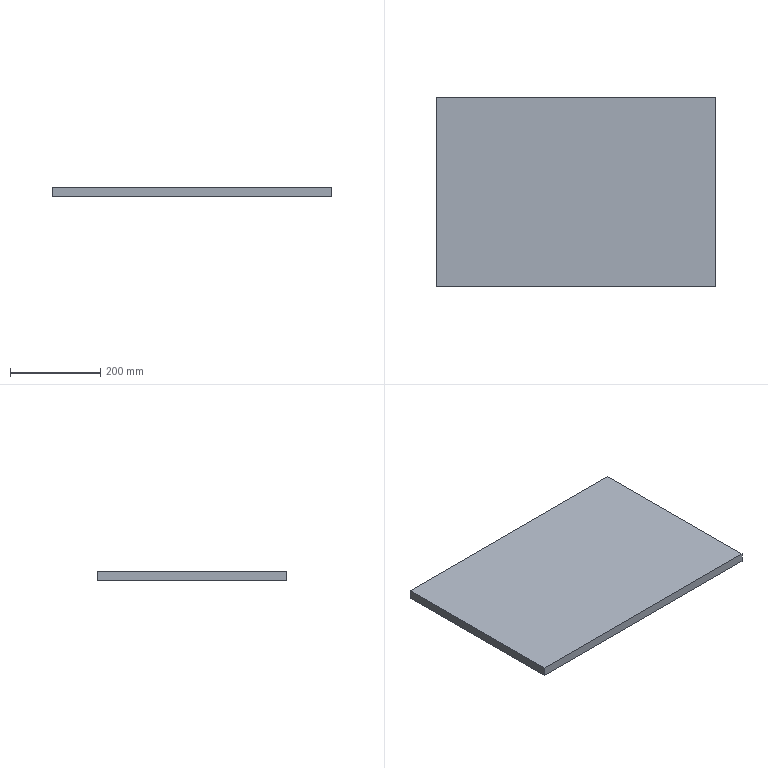Part | STEP file | Pad plate 2 | 1 solid | 6 faces | box 620 x 420 x 20 mm | volume 5208000 mm3 | plane 6
STEP:
#1=CARTESIAN_POINT('',(0.,0.,0.));
#2=DIRECTION('',(0.,0.,1.));
#3=DIRECTION('',(1.,0.,0.));
#4=AXIS2_PLACEMENT_3D('',#1,#2,#3);
#5=CARTESIAN_POINT('',(-310.,210.,20.));
#6=VERTEX_POINT('',#5);
#7=CARTESIAN_POINT('',(-310.,-210.,20.));
#8=VERTEX_POINT('',#7);
#9=CARTESIAN_POINT('',(-310.,0.,20.));
#10=DIRECTION('',(0.,-1.,0.));
#11=VECTOR('',#10,1.);
#12=LINE('',#9,#11);
#13=CARTESIAN_POINT('',(0.,0.,20.));
#14=DIRECTION('',(0.,0.,1.));
#15=DIRECTION('',(1.,0.,0.));
#16=AXIS2_PLACEMENT_3D('',#13,#14,#15);
#17=PLANE('',#16);
#18=CARTESIAN_POINT('',(-310.,0.));
#19=DIRECTION('',(0.,-1.));
#20=VECTOR('',#19,1.);
#21=LINE('',#18,#20);
#22=(GEOMETRIC_REPRESENTATION_CONTEXT(2)PARAMETRIC_REPRESENTATION_CONTEXT()REPRESENTATION_CONTEXT('',''));
#23=DEFINITIONAL_REPRESENTATION('',(#21),#22);
#24=PCURVE('',#17,#23);
#25=CARTESIAN_POINT('',(-310.,210.,20.));
#26=DIRECTION('',(1.,0.,0.));
#27=DIRECTION('',(0.,1.,0.));
#28=AXIS2_PLACEMENT_3D('',#25,#26,#27);
#29=PLANE('',#28);
#30=CARTESIAN_POINT('',(-210.,0.));
#31=DIRECTION('',(-1.,0.));
#32=VECTOR('',#31,1.);
#33=LINE('',#30,#32);
#34=(GEOMETRIC_REPRESENTATION_CONTEXT(2)PARAMETRIC_REPRESENTATION_CONTEXT()REPRESENTATION_CONTEXT('',''));
#35=DEFINITIONAL_REPRESENTATION('',(#33),#34);
#36=PCURVE('',#29,#35);
#37=SURFACE_CURVE('',#12,(#24,#36),.PCURVE_S1.);
#38=EDGE_CURVE('',#6,#8,#37,.T.);
#39=ORIENTED_EDGE('',*,*,#38,.T.);
#40=CARTESIAN_POINT('',(310.,-210.,20.));
#41=VERTEX_POINT('',#40);
#42=CARTESIAN_POINT('',(0.,-210.,20.));
#43=DIRECTION('',(1.,0.,0.));
#44=VECTOR('',#43,1.);
#45=LINE('',#42,#44);
#46=CARTESIAN_POINT('',(0.,-210.));
#47=DIRECTION('',(1.,0.));
#48=VECTOR('',#47,1.);
#49=LINE('',#46,#48);
#50=(GEOMETRIC_REPRESENTATION_CONTEXT(2)PARAMETRIC_REPRESENTATION_CONTEXT()REPRESENTATION_CONTEXT('',''));
#51=DEFINITIONAL_REPRESENTATION('',(#49),#50);
#52=PCURVE('',#17,#51);
#53=CARTESIAN_POINT('',(-310.,-210.,20.));
#54=DIRECTION('',(0.,1.,0.));
#55=DIRECTION('',(0.,0.,1.));
#56=AXIS2_PLACEMENT_3D('',#53,#54,#55);
#57=PLANE('',#56);
#58=CARTESIAN_POINT('',(0.,310.));
#59=DIRECTION('',(0.,1.));
#60=VECTOR('',#59,1.);
#61=LINE('',#58,#60);
#62=(GEOMETRIC_REPRESENTATION_CONTEXT(2)PARAMETRIC_REPRESENTATION_CONTEXT()REPRESENTATION_CONTEXT('',''));
#63=DEFINITIONAL_REPRESENTATION('',(#61),#62);
#64=PCURVE('',#57,#63);
#65=SURFACE_CURVE('',#45,(#52,#64),.PCURVE_S1.);
#66=EDGE_CURVE('',#8,#41,#65,.T.);
#67=ORIENTED_EDGE('',*,*,#66,.T.);
#68=CARTESIAN_POINT('',(310.,210.,20.));
#69=VERTEX_POINT('',#68);
#70=CARTESIAN_POINT('',(310.,0.,20.));
#71=DIRECTION('',(0.,1.,0.));
#72=VECTOR('',#71,1.);
#73=LINE('',#70,#72);
#74=CARTESIAN_POINT('',(310.,0.));
#75=DIRECTION('',(0.,1.));
#76=VECTOR('',#75,1.);
#77=LINE('',#74,#76);
#78=(GEOMETRIC_REPRESENTATION_CONTEXT(2)PARAMETRIC_REPRESENTATION_CONTEXT()REPRESENTATION_CONTEXT('',''));
#79=DEFINITIONAL_REPRESENTATION('',(#77),#78);
#80=PCURVE('',#17,#79);
#81=CARTESIAN_POINT('',(310.,210.,20.));
#82=DIRECTION('',(-1.,0.,0.));
#83=DIRECTION('',(0.,0.,1.));
#84=AXIS2_PLACEMENT_3D('',#81,#82,#83);
#85=PLANE('',#84);
#86=CARTESIAN_POINT('',(0.,-210.));
#87=DIRECTION('',(0.,1.));
#88=VECTOR('',#87,1.);
#89=LINE('',#86,#88);
#90=(GEOMETRIC_REPRESENTATION_CONTEXT(2)PARAMETRIC_REPRESENTATION_CONTEXT()REPRESENTATION_CONTEXT('',''));
#91=DEFINITIONAL_REPRESENTATION('',(#89),#90);
#92=PCURVE('',#85,#91);
#93=SURFACE_CURVE('',#73,(#80,#92),.PCURVE_S1.);
#94=EDGE_CURVE('',#41,#69,#93,.T.);
#95=ORIENTED_EDGE('',*,*,#94,.T.);
#96=CARTESIAN_POINT('',(0.,210.,20.));
#97=DIRECTION('',(-1.,0.,0.));
#98=VECTOR('',#97,1.);
#99=LINE('',#96,#98);
#100=CARTESIAN_POINT('',(0.,210.));
#101=DIRECTION('',(-1.,0.));
#102=VECTOR('',#101,1.);
#103=LINE('',#100,#102);
#104=(GEOMETRIC_REPRESENTATION_CONTEXT(2)PARAMETRIC_REPRESENTATION_CONTEXT()REPRESENTATION_CONTEXT('',''));
#105=DEFINITIONAL_REPRESENTATION('',(#103),#104);
#106=PCURVE('',#17,#105);
#107=CARTESIAN_POINT('',(-310.,210.,20.));
#108=DIRECTION('',(0.,-1.,0.));
#109=DIRECTION('',(0.,0.,-1.));
#110=AXIS2_PLACEMENT_3D('',#107,#108,#109);
#111=PLANE('',#110);
#112=CARTESIAN_POINT('',(0.,310.));
#113=DIRECTION('',(0.,-1.));
#114=VECTOR('',#113,1.);
#115=LINE('',#112,#114);
#116=(GEOMETRIC_REPRESENTATION_CONTEXT(2)PARAMETRIC_REPRESENTATION_CONTEXT()REPRESENTATION_CONTEXT('',''));
#117=DEFINITIONAL_REPRESENTATION('',(#115),#116);
#118=PCURVE('',#111,#117);
#119=SURFACE_CURVE('',#99,(#106,#118),.PCURVE_S1.);
#120=EDGE_CURVE('',#69,#6,#119,.T.);
#121=ORIENTED_EDGE('',*,*,#120,.T.);
#122=EDGE_LOOP('',(#39,#67,#95,#121));
#123=FACE_BOUND('',#122,.T.);
#124=ADVANCED_FACE('',(#123),#17,.T.);
#125=CARTESIAN_POINT('',(310.,-210.,0.));
#126=VERTEX_POINT('',#125);
#127=CARTESIAN_POINT('',(310.,-210.,20.));
#128=DIRECTION('',(0.,0.,-1.));
#129=VECTOR('',#128,1.);
#130=LINE('',#127,#129);
#131=CARTESIAN_POINT('',(0.,620.));
#132=DIRECTION('',(-1.,0.));
#133=VECTOR('',#132,1.);
#134=LINE('',#131,#133);
#135=(GEOMETRIC_REPRESENTATION_CONTEXT(2)PARAMETRIC_REPRESENTATION_CONTEXT()REPRESENTATION_CONTEXT('',''));
#136=DEFINITIONAL_REPRESENTATION('',(#134),#135);
#137=PCURVE('',#57,#136);
#138=CARTESIAN_POINT('',(0.,-420.));
#139=DIRECTION('',(-1.,0.));
#140=VECTOR('',#139,1.);
#141=LINE('',#138,#140);
#142=(GEOMETRIC_REPRESENTATION_CONTEXT(2)PARAMETRIC_REPRESENTATION_CONTEXT()REPRESENTATION_CONTEXT('',''));
#143=DEFINITIONAL_REPRESENTATION('',(#141),#142);
#144=PCURVE('',#85,#143);
#145=SURFACE_CURVE('',#130,(#137,#144),.PCURVE_S1.);
#146=EDGE_CURVE('',#41,#126,#145,.T.);
#147=ORIENTED_EDGE('',*,*,#146,.F.);
#148=ORIENTED_EDGE('',*,*,#66,.F.);
#149=CARTESIAN_POINT('',(-310.,-210.,0.));
#150=VERTEX_POINT('',#149);
#151=CARTESIAN_POINT('',(-310.,-210.,20.));
#152=DIRECTION('',(0.,0.,1.));
#153=VECTOR('',#152,1.);
#154=LINE('',#151,#153);
#155=CARTESIAN_POINT('',(0.,0.));
#156=DIRECTION('',(1.,0.));
#157=VECTOR('',#156,1.);
#158=LINE('',#155,#157);
#159=(GEOMETRIC_REPRESENTATION_CONTEXT(2)PARAMETRIC_REPRESENTATION_CONTEXT()REPRESENTATION_CONTEXT('',''));
#160=DEFINITIONAL_REPRESENTATION('',(#158),#159);
#161=PCURVE('',#57,#160);
#162=CARTESIAN_POINT('',(-420.,0.));
#163=DIRECTION('',(0.,1.));
#164=VECTOR('',#163,1.);
#165=LINE('',#162,#164);
#166=(GEOMETRIC_REPRESENTATION_CONTEXT(2)PARAMETRIC_REPRESENTATION_CONTEXT()REPRESENTATION_CONTEXT('',''));
#167=DEFINITIONAL_REPRESENTATION('',(#165),#166);
#168=PCURVE('',#29,#167);
#169=SURFACE_CURVE('',#154,(#161,#168),.PCURVE_S1.);
#170=EDGE_CURVE('',#150,#8,#169,.T.);
#171=ORIENTED_EDGE('',*,*,#170,.F.);
#172=CARTESIAN_POINT('',(-310.,-210.,0.));
#173=DIRECTION('',(-1.,0.,0.));
#174=VECTOR('',#173,1.);
#175=LINE('',#172,#174);
#176=CARTESIAN_POINT('',(-20.,0.));
#177=DIRECTION('',(0.,-1.));
#178=VECTOR('',#177,1.);
#179=LINE('',#176,#178);
#180=(GEOMETRIC_REPRESENTATION_CONTEXT(2)PARAMETRIC_REPRESENTATION_CONTEXT()REPRESENTATION_CONTEXT('',''));
#181=DEFINITIONAL_REPRESENTATION('',(#179),#180);
#182=PCURVE('',#57,#181);
#183=CARTESIAN_POINT('',(0.,0.,0.));
#184=DIRECTION('',(0.,0.,1.));
#185=DIRECTION('',(1.,0.,0.));
#186=AXIS2_PLACEMENT_3D('',#183,#184,#185);
#187=PLANE('',#186);
#188=CARTESIAN_POINT('',(-310.,-210.));
#189=DIRECTION('',(-1.,0.));
#190=VECTOR('',#189,1.);
#191=LINE('',#188,#190);
#192=(GEOMETRIC_REPRESENTATION_CONTEXT(2)PARAMETRIC_REPRESENTATION_CONTEXT()REPRESENTATION_CONTEXT('',''));
#193=DEFINITIONAL_REPRESENTATION('',(#191),#192);
#194=PCURVE('',#187,#193);
#195=SURFACE_CURVE('',#175,(#182,#194),.PCURVE_S1.);
#196=EDGE_CURVE('',#126,#150,#195,.T.);
#197=ORIENTED_EDGE('',*,*,#196,.F.);
#198=EDGE_LOOP('',(#147,#148,#171,#197));
#199=FACE_BOUND('',#198,.T.);
#200=ADVANCED_FACE('',(#199),#57,.F.);
#201=ORIENTED_EDGE('',*,*,#170,.T.);
#202=ORIENTED_EDGE('',*,*,#38,.F.);
#203=CARTESIAN_POINT('',(-310.,210.,0.));
#204=VERTEX_POINT('',#203);
#205=CARTESIAN_POINT('',(-310.,210.,20.));
#206=DIRECTION('',(0.,0.,1.));
#207=VECTOR('',#206,1.);
#208=LINE('',#205,#207);
#209=CARTESIAN_POINT('',(0.,0.));
#210=DIRECTION('',(0.,1.));
#211=VECTOR('',#210,1.);
#212=LINE('',#209,#211);
#213=(GEOMETRIC_REPRESENTATION_CONTEXT(2)PARAMETRIC_REPRESENTATION_CONTEXT()REPRESENTATION_CONTEXT('',''));
#214=DEFINITIONAL_REPRESENTATION('',(#212),#213);
#215=PCURVE('',#29,#214);
#216=CARTESIAN_POINT('',(0.,0.));
#217=DIRECTION('',(-1.,0.));
#218=VECTOR('',#217,1.);
#219=LINE('',#216,#218);
#220=(GEOMETRIC_REPRESENTATION_CONTEXT(2)PARAMETRIC_REPRESENTATION_CONTEXT()REPRESENTATION_CONTEXT('',''));
#221=DEFINITIONAL_REPRESENTATION('',(#219),#220);
#222=PCURVE('',#111,#221);
#223=SURFACE_CURVE('',#208,(#215,#222),.PCURVE_S1.);
#224=EDGE_CURVE('',#204,#6,#223,.T.);
#225=ORIENTED_EDGE('',*,*,#224,.F.);
#226=CARTESIAN_POINT('',(-310.,210.,0.));
#227=DIRECTION('',(0.,1.,0.));
#228=VECTOR('',#227,1.);
#229=LINE('',#226,#228);
#230=CARTESIAN_POINT('',(0.,-20.));
#231=DIRECTION('',(1.,0.));
#232=VECTOR('',#231,1.);
#233=LINE('',#230,#232);
#234=(GEOMETRIC_REPRESENTATION_CONTEXT(2)PARAMETRIC_REPRESENTATION_CONTEXT()REPRESENTATION_CONTEXT('',''));
#235=DEFINITIONAL_REPRESENTATION('',(#233),#234);
#236=PCURVE('',#29,#235);
#237=CARTESIAN_POINT('',(-310.,210.));
#238=DIRECTION('',(0.,1.));
#239=VECTOR('',#238,1.);
#240=LINE('',#237,#239);
#241=(GEOMETRIC_REPRESENTATION_CONTEXT(2)PARAMETRIC_REPRESENTATION_CONTEXT()REPRESENTATION_CONTEXT('',''));
#242=DEFINITIONAL_REPRESENTATION('',(#240),#241);
#243=PCURVE('',#187,#242);
#244=SURFACE_CURVE('',#229,(#236,#243),.PCURVE_S1.);
#245=EDGE_CURVE('',#150,#204,#244,.T.);
#246=ORIENTED_EDGE('',*,*,#245,.F.);
#247=EDGE_LOOP('',(#201,#202,#225,#246));
#248=FACE_BOUND('',#247,.T.);
#249=ADVANCED_FACE('',(#248),#29,.F.);
#250=ORIENTED_EDGE('',*,*,#224,.T.);
#251=ORIENTED_EDGE('',*,*,#120,.F.);
#252=CARTESIAN_POINT('',(310.,210.,0.));
#253=VERTEX_POINT('',#252);
#254=CARTESIAN_POINT('',(310.,210.,20.));
#255=DIRECTION('',(0.,0.,1.));
#256=VECTOR('',#255,1.);
#257=LINE('',#254,#256);
#258=CARTESIAN_POINT('',(0.,620.));
#259=DIRECTION('',(-1.,0.));
#260=VECTOR('',#259,1.);
#261=LINE('',#258,#260);
#262=(GEOMETRIC_REPRESENTATION_CONTEXT(2)PARAMETRIC_REPRESENTATION_CONTEXT()REPRESENTATION_CONTEXT('',''));
#263=DEFINITIONAL_REPRESENTATION('',(#261),#262);
#264=PCURVE('',#111,#263);
#265=CARTESIAN_POINT('',(0.,0.));
#266=DIRECTION('',(1.,0.));
#267=VECTOR('',#266,1.);
#268=LINE('',#265,#267);
#269=(GEOMETRIC_REPRESENTATION_CONTEXT(2)PARAMETRIC_REPRESENTATION_CONTEXT()REPRESENTATION_CONTEXT('',''));
#270=DEFINITIONAL_REPRESENTATION('',(#268),#269);
#271=PCURVE('',#85,#270);
#272=SURFACE_CURVE('',#257,(#264,#271),.PCURVE_S1.);
#273=EDGE_CURVE('',#253,#69,#272,.T.);
#274=ORIENTED_EDGE('',*,*,#273,.F.);
#275=CARTESIAN_POINT('',(-310.,210.,0.));
#276=DIRECTION('',(1.,0.,0.));
#277=VECTOR('',#276,1.);
#278=LINE('',#275,#277);
#279=CARTESIAN_POINT('',(20.,0.));
#280=DIRECTION('',(0.,1.));
#281=VECTOR('',#280,1.);
#282=LINE('',#279,#281);
#283=(GEOMETRIC_REPRESENTATION_CONTEXT(2)PARAMETRIC_REPRESENTATION_CONTEXT()REPRESENTATION_CONTEXT('',''));
#284=DEFINITIONAL_REPRESENTATION('',(#282),#283);
#285=PCURVE('',#111,#284);
#286=CARTESIAN_POINT('',(-310.,210.));
#287=DIRECTION('',(1.,0.));
#288=VECTOR('',#287,1.);
#289=LINE('',#286,#288);
#290=(GEOMETRIC_REPRESENTATION_CONTEXT(2)PARAMETRIC_REPRESENTATION_CONTEXT()REPRESENTATION_CONTEXT('',''));
#291=DEFINITIONAL_REPRESENTATION('',(#289),#290);
#292=PCURVE('',#187,#291);
#293=SURFACE_CURVE('',#278,(#285,#292),.PCURVE_S1.);
#294=EDGE_CURVE('',#204,#253,#293,.T.);
#295=ORIENTED_EDGE('',*,*,#294,.F.);
#296=EDGE_LOOP('',(#250,#251,#274,#295));
#297=FACE_BOUND('',#296,.T.);
#298=ADVANCED_FACE('',(#297),#111,.F.);
#299=ORIENTED_EDGE('',*,*,#273,.T.);
#300=ORIENTED_EDGE('',*,*,#94,.F.);
#301=ORIENTED_EDGE('',*,*,#146,.T.);
#302=CARTESIAN_POINT('',(310.,210.,0.));
#303=DIRECTION('',(0.,-1.,0.));
#304=VECTOR('',#303,1.);
#305=LINE('',#302,#304);
#306=CARTESIAN_POINT('',(-20.,0.));
#307=DIRECTION('',(0.,-1.));
#308=VECTOR('',#307,1.);
#309=LINE('',#306,#308);
#310=(GEOMETRIC_REPRESENTATION_CONTEXT(2)PARAMETRIC_REPRESENTATION_CONTEXT()REPRESENTATION_CONTEXT('',''));
#311=DEFINITIONAL_REPRESENTATION('',(#309),#310);
#312=PCURVE('',#85,#311);
#313=CARTESIAN_POINT('',(310.,210.));
#314=DIRECTION('',(0.,-1.));
#315=VECTOR('',#314,1.);
#316=LINE('',#313,#315);
#317=(GEOMETRIC_REPRESENTATION_CONTEXT(2)PARAMETRIC_REPRESENTATION_CONTEXT()REPRESENTATION_CONTEXT('',''));
#318=DEFINITIONAL_REPRESENTATION('',(#316),#317);
#319=PCURVE('',#187,#318);
#320=SURFACE_CURVE('',#305,(#312,#319),.PCURVE_S1.);
#321=EDGE_CURVE('',#253,#126,#320,.T.);
#322=ORIENTED_EDGE('',*,*,#321,.F.);
#323=EDGE_LOOP('',(#299,#300,#301,#322));
#324=FACE_BOUND('',#323,.T.);
#325=ADVANCED_FACE('',(#324),#85,.F.);
#326=ORIENTED_EDGE('',*,*,#196,.T.);
#327=ORIENTED_EDGE('',*,*,#245,.T.);
#328=ORIENTED_EDGE('',*,*,#294,.T.);
#329=ORIENTED_EDGE('',*,*,#321,.T.);
#330=EDGE_LOOP('',(#326,#327,#328,#329));
#331=FACE_BOUND('',#330,.T.);
#332=ADVANCED_FACE('',(#331),#187,.F.);
#333=CLOSED_SHELL('',(#124,#200,#249,#298,#325,#332));
#334=MANIFOLD_SOLID_BREP('',#333);
#335=(LENGTH_UNIT()NAMED_UNIT(*)SI_UNIT(.MILLI.,.METRE.));
#336=UNCERTAINTY_MEASURE_WITH_UNIT(LENGTH_MEASURE(0.0000001),#335,'','');
#337=(NAMED_UNIT(*)PLANE_ANGLE_UNIT()SI_UNIT($,.RADIAN.));
#338=(NAMED_UNIT(*)SI_UNIT($,.STERADIAN.)SOLID_ANGLE_UNIT());
#339=(GEOMETRIC_REPRESENTATION_CONTEXT(3)GLOBAL_UNCERTAINTY_ASSIGNED_CONTEXT((#336))GLOBAL_UNIT_ASSIGNED_CONTEXT((#335,#337,#338))REPRESENTATION_CONTEXT('',''));
#340=ADVANCED_BREP_SHAPE_REPRESENTATION('',(#4,#334),#339);